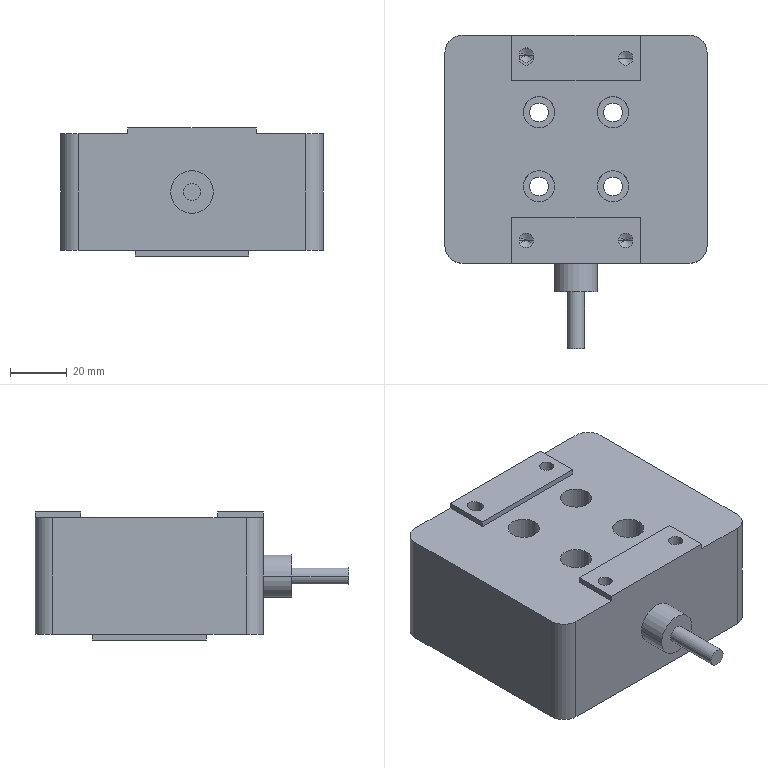Part | SolidWorks | features ICE 6, Extrusion 1, Fillet 1, HoleWzd 1 | 1 solid | 69 faces | box 92 x 110 x 45 mm | volume 294451 mm3 | cylinder 35 | plane 26 | cone 8 | commonest cylinder face diameters 5 x11 6.6 x8 11 x8 12 x4 6 x2 15 x2